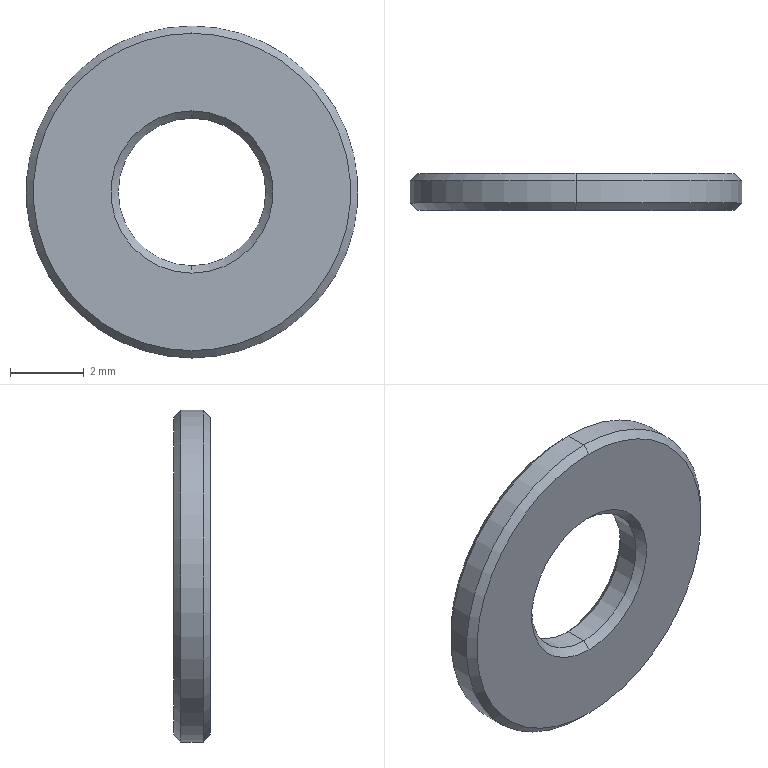Part | NX | features BREP 1 | 1 solid | 14 faces | box 9 x 1 x 9 mm | volume 49.417 mm3 | cone 8 | cylinder 4 | plane 2 | commonest cylinder face diameters 4 x2 9 x2
STEP:
#1=CARTESIAN_POINT('',(0.,1.,4.3));
#2=VERTEX_POINT('',#1);
#3=CARTESIAN_POINT('',(0.,1.,-4.3));
#4=VERTEX_POINT('',#3);
#5=CARTESIAN_POINT('',(0.,1.,0.));
#6=DIRECTION('',(0.,1.,0.));
#7=DIRECTION('',(1.,0.,0.));
#8=AXIS2_PLACEMENT_3D('',#5,#6,#7);
#9=CIRCLE('',#8,4.3);
#10=EDGE_CURVE('',#2,#4,#9,.T.);
#11=ORIENTED_EDGE('',*,*,#10,.F.);
#12=CARTESIAN_POINT('',(0.,0.8,4.5));
#13=VERTEX_POINT('',#12);
#14=CARTESIAN_POINT('',(0.,-353550.241,353555.541));
#15=DIRECTION('',(0.,0.7071,-0.7071));
#16=VECTOR('',#15,1000.);
#17=LINE('',#14,#16);
#18=EDGE_CURVE('',#13,#2,#17,.T.);
#19=ORIENTED_EDGE('',*,*,#18,.F.);
#20=CARTESIAN_POINT('',(0.,0.8,-4.5));
#21=VERTEX_POINT('',#20);
#22=CARTESIAN_POINT('',(0.,0.8,0.));
#23=DIRECTION('',(0.,-1.,0.));
#24=DIRECTION('',(1.,0.,0.));
#25=AXIS2_PLACEMENT_3D('',#22,#23,#24);
#26=CIRCLE('',#25,4.5);
#27=EDGE_CURVE('',#21,#13,#26,.T.);
#28=ORIENTED_EDGE('',*,*,#27,.F.);
#29=CARTESIAN_POINT('',(0.,-353550.241,-353555.541));
#30=DIRECTION('',(0.,0.7071,0.7071));
#31=VECTOR('',#30,1000.);
#32=LINE('',#29,#31);
#33=EDGE_CURVE('',#21,#4,#32,.T.);
#34=ORIENTED_EDGE('',*,*,#33,.T.);
#35=EDGE_LOOP('',(#11,#19,#28,#34));
#36=FACE_BOUND('',#35,.T.);
#37=CARTESIAN_POINT('',(0.,1.,0.));
#38=DIRECTION('',(0.,-1.,0.));
#39=DIRECTION('',(0.,0.,1.));
#40=AXIS2_PLACEMENT_3D('',#37,#38,#39);
#41=CONICAL_SURFACE('',#40,4.3,0.7854);
#42=ADVANCED_FACE('',(#36),#41,.T.);
#43=CARTESIAN_POINT('',(0.,1.,0.));
#44=DIRECTION('',(0.,1.,0.));
#45=DIRECTION('',(1.,0.,0.));
#46=AXIS2_PLACEMENT_3D('',#43,#44,#45);
#47=CIRCLE('',#46,4.3);
#48=EDGE_CURVE('',#4,#2,#47,.T.);
#49=ORIENTED_EDGE('',*,*,#48,.T.);
#50=ORIENTED_EDGE('',*,*,#10,.T.);
#51=EDGE_LOOP('',(#49,#50));
#52=FACE_BOUND('',#51,.T.);
#53=CARTESIAN_POINT('',(0.,1.,2.2));
#54=VERTEX_POINT('',#53);
#55=CARTESIAN_POINT('',(0.,1.,-2.2));
#56=VERTEX_POINT('',#55);
#57=CARTESIAN_POINT('',(0.,1.,2.2));
#58=CARTESIAN_POINT('',(-0.218,1.,2.2));
#59=CARTESIAN_POINT('',(-0.436,1.,2.173));
#60=CARTESIAN_POINT('',(-0.6495,1.,2.119));
#61=CARTESIAN_POINT('',(-1.059,1.,1.959));
#62=CARTESIAN_POINT('',(-1.417,1.,1.704));
#63=CARTESIAN_POINT('',(-1.579,1.,1.555));
#64=CARTESIAN_POINT('',(-1.863,1.,1.22));
#65=CARTESIAN_POINT('',(-2.057,1.,0.826));
#66=CARTESIAN_POINT('',(-2.128,1.,0.6178));
#67=CARTESIAN_POINT('',(-2.219,1.,0.1879));
#68=CARTESIAN_POINT('',(-2.202,1.,-0.251));
#69=CARTESIAN_POINT('',(-2.166,1.,-0.4684));
#70=CARTESIAN_POINT('',(-2.042,1.,-0.8896));
#71=CARTESIAN_POINT('',(-1.818,1.,-1.268));
#72=CARTESIAN_POINT('',(-1.683,1.,-1.442));
#73=CARTESIAN_POINT('',(-1.373,1.,-1.753));
#74=CARTESIAN_POINT('',(-0.9967,1.,-1.98));
#75=CARTESIAN_POINT('',(-0.7952,1.,-2.069));
#76=CARTESIAN_POINT('',(-0.5132,1.,-2.154));
#77=CARTESIAN_POINT('',(-0.223,1.,-2.191));
#78=CARTESIAN_POINT('',(-0.1486,1.,-2.197));
#79=CARTESIAN_POINT('',(-0.07431,1.,-2.2));
#80=CARTESIAN_POINT('',(0.,1.,-2.2));
#81=B_SPLINE_CURVE_WITH_KNOTS('',5,(#57,#58,#59,#60,#61,#62,#63,#64,#65,#66,#67,#68,#69,#70,#71,#72,#73,#74,#75,#76,#77,#78,#79,#80),.UNSPECIFIED.,.F.,.F.,(6,3,3,3,3,3,3,6),(0.,0.1577,0.3154,0.4731,0.6308,0.7885,0.9462,1.),.UNSPECIFIED.);
#82=EDGE_CURVE('',#54,#56,#81,.T.);
#83=ORIENTED_EDGE('',*,*,#82,.T.);
#84=CARTESIAN_POINT('',(0.,1.,-2.2));
#85=CARTESIAN_POINT('',(0.218,1.,-2.2));
#86=CARTESIAN_POINT('',(0.436,1.,-2.173));
#87=CARTESIAN_POINT('',(0.6495,1.,-2.119));
#88=CARTESIAN_POINT('',(1.059,1.,-1.959));
#89=CARTESIAN_POINT('',(1.417,1.,-1.704));
#90=CARTESIAN_POINT('',(1.579,1.,-1.555));
#91=CARTESIAN_POINT('',(1.863,1.,-1.22));
#92=CARTESIAN_POINT('',(2.057,1.,-0.826));
#93=CARTESIAN_POINT('',(2.128,1.,-0.6178));
#94=CARTESIAN_POINT('',(2.219,1.,-0.1879));
#95=CARTESIAN_POINT('',(2.202,1.,0.251));
#96=CARTESIAN_POINT('',(2.166,1.,0.4684));
#97=CARTESIAN_POINT('',(2.042,1.,0.8896));
#98=CARTESIAN_POINT('',(1.818,1.,1.268));
#99=CARTESIAN_POINT('',(1.683,1.,1.442));
#100=CARTESIAN_POINT('',(1.373,1.,1.753));
#101=CARTESIAN_POINT('',(0.9967,1.,1.98));
#102=CARTESIAN_POINT('',(0.7952,1.,2.069));
#103=CARTESIAN_POINT('',(0.5132,1.,2.154));
#104=CARTESIAN_POINT('',(0.223,1.,2.191));
#105=CARTESIAN_POINT('',(0.1486,1.,2.197));
#106=CARTESIAN_POINT('',(0.07431,1.,2.2));
#107=CARTESIAN_POINT('',(0.,1.,2.2));
#108=B_SPLINE_CURVE_WITH_KNOTS('',5,(#84,#85,#86,#87,#88,#89,#90,#91,#92,#93,#94,#95,#96,#97,#98,#99,#100,#101,#102,#103,#104,#105,#106,#107),.UNSPECIFIED.,.F.,.F.,(6,3,3,3,3,3,3,6),(0.,0.1577,0.3154,0.4731,0.6308,0.7885,0.9462,1.),.UNSPECIFIED.);
#109=EDGE_CURVE('',#56,#54,#108,.T.);
#110=ORIENTED_EDGE('',*,*,#109,.T.);
#111=EDGE_LOOP('',(#83,#110));
#112=FACE_BOUND('',#111,.T.);
#113=CARTESIAN_POINT('',(0.,1.,0.));
#114=DIRECTION('',(0.,1.,0.));
#115=DIRECTION('',(0.,0.,-1.));
#116=AXIS2_PLACEMENT_3D('',#113,#114,#115);
#117=PLANE('',#116);
#118=ADVANCED_FACE('',(#52,#112),#117,.T.);
#119=ORIENTED_EDGE('',*,*,#18,.T.);
#120=ORIENTED_EDGE('',*,*,#48,.F.);
#121=ORIENTED_EDGE('',*,*,#33,.F.);
#122=CARTESIAN_POINT('',(0.,0.8,0.));
#123=DIRECTION('',(0.,-1.,0.));
#124=DIRECTION('',(1.,0.,0.));
#125=AXIS2_PLACEMENT_3D('',#122,#123,#124);
#126=CIRCLE('',#125,4.5);
#127=EDGE_CURVE('',#13,#21,#126,.T.);
#128=ORIENTED_EDGE('',*,*,#127,.F.);
#129=EDGE_LOOP('',(#119,#120,#121,#128));
#130=FACE_BOUND('',#129,.T.);
#131=CARTESIAN_POINT('',(0.,1.,0.));
#132=DIRECTION('',(0.,-1.,0.));
#133=DIRECTION('',(0.,0.,-1.));
#134=AXIS2_PLACEMENT_3D('',#131,#132,#133);
#135=CONICAL_SURFACE('',#134,4.3,0.7854);
#136=ADVANCED_FACE('',(#130),#135,.T.);
#137=ORIENTED_EDGE('',*,*,#27,.T.);
#138=CARTESIAN_POINT('',(0.,0.2,4.5));
#139=VERTEX_POINT('',#138);
#140=CARTESIAN_POINT('',(0.,1.,4.5));
#141=DIRECTION('',(0.,1.,0.));
#142=VECTOR('',#141,1000.);
#143=LINE('',#140,#142);
#144=EDGE_CURVE('',#139,#13,#143,.T.);
#145=ORIENTED_EDGE('',*,*,#144,.F.);
#146=CARTESIAN_POINT('',(0.,0.2,-4.5));
#147=VERTEX_POINT('',#146);
#148=CARTESIAN_POINT('',(0.,0.2,0.));
#149=DIRECTION('',(0.,1.,0.));
#150=DIRECTION('',(1.,0.,0.));
#151=AXIS2_PLACEMENT_3D('',#148,#149,#150);
#152=CIRCLE('',#151,4.5);
#153=EDGE_CURVE('',#139,#147,#152,.T.);
#154=ORIENTED_EDGE('',*,*,#153,.T.);
#155=CARTESIAN_POINT('',(0.,1.,-4.5));
#156=DIRECTION('',(0.,1.,0.));
#157=VECTOR('',#156,1000.);
#158=LINE('',#155,#157);
#159=EDGE_CURVE('',#147,#21,#158,.T.);
#160=ORIENTED_EDGE('',*,*,#159,.T.);
#161=EDGE_LOOP('',(#137,#145,#154,#160));
#162=FACE_BOUND('',#161,.T.);
#163=CARTESIAN_POINT('',(0.,1.,0.));
#164=DIRECTION('',(0.,-1.,0.));
#165=DIRECTION('',(0.,0.,1.));
#166=AXIS2_PLACEMENT_3D('',#163,#164,#165);
#167=CYLINDRICAL_SURFACE('',#166,4.5);
#168=ADVANCED_FACE('',(#162),#167,.T.);
#169=CARTESIAN_POINT('',(0.,0.8,-2.));
#170=VERTEX_POINT('',#169);
#171=CARTESIAN_POINT('',(0.,0.8,2.));
#172=VERTEX_POINT('',#171);
#173=CARTESIAN_POINT('',(0.,0.8,0.));
#174=DIRECTION('',(0.,1.,0.));
#175=DIRECTION('',(1.,0.,0.));
#176=AXIS2_PLACEMENT_3D('',#173,#174,#175);
#177=CIRCLE('',#176,2.);
#178=EDGE_CURVE('',#170,#172,#177,.T.);
#179=ORIENTED_EDGE('',*,*,#178,.F.);
#180=CARTESIAN_POINT('',(0.,353553.191,-353554.391));
#181=DIRECTION('',(0.,0.7071,-0.7071));
#182=VECTOR('',#181,1000.);
#183=LINE('',#180,#182);
#184=EDGE_CURVE('',#170,#56,#183,.T.);
#185=ORIENTED_EDGE('',*,*,#184,.T.);
#186=ORIENTED_EDGE('',*,*,#82,.F.);
#187=CARTESIAN_POINT('',(0.,353553.191,353554.391));
#188=DIRECTION('',(0.,0.7071,0.7071));
#189=VECTOR('',#188,1000.);
#190=LINE('',#187,#189);
#191=EDGE_CURVE('',#172,#54,#190,.T.);
#192=ORIENTED_EDGE('',*,*,#191,.F.);
#193=EDGE_LOOP('',(#179,#185,#186,#192));
#194=FACE_BOUND('',#193,.T.);
#195=CARTESIAN_POINT('',(0.,0.8,0.));
#196=DIRECTION('',(0.,1.,0.));
#197=DIRECTION('',(0.,0.,1.));
#198=AXIS2_PLACEMENT_3D('',#195,#196,#197);
#199=CONICAL_SURFACE('',#198,2.,0.7854);
#200=ADVANCED_FACE('',(#194),#199,.F.);
#201=ORIENTED_EDGE('',*,*,#184,.F.);
#202=CARTESIAN_POINT('',(0.,0.8,0.));
#203=DIRECTION('',(0.,1.,0.));
#204=DIRECTION('',(1.,0.,0.));
#205=AXIS2_PLACEMENT_3D('',#202,#203,#204);
#206=CIRCLE('',#205,2.);
#207=EDGE_CURVE('',#172,#170,#206,.T.);
#208=ORIENTED_EDGE('',*,*,#207,.F.);
#209=ORIENTED_EDGE('',*,*,#191,.T.);
#210=ORIENTED_EDGE('',*,*,#109,.F.);
#211=EDGE_LOOP('',(#201,#208,#209,#210));
#212=FACE_BOUND('',#211,.T.);
#213=CARTESIAN_POINT('',(0.,0.8,0.));
#214=DIRECTION('',(0.,1.,0.));
#215=DIRECTION('',(0.,0.,-1.));
#216=AXIS2_PLACEMENT_3D('',#213,#214,#215);
#217=CONICAL_SURFACE('',#216,2.,0.7854);
#218=ADVANCED_FACE('',(#212),#217,.F.);
#219=ORIENTED_EDGE('',*,*,#144,.T.);
#220=ORIENTED_EDGE('',*,*,#127,.T.);
#221=ORIENTED_EDGE('',*,*,#159,.F.);
#222=CARTESIAN_POINT('',(0.,0.2,0.));
#223=DIRECTION('',(0.,1.,0.));
#224=DIRECTION('',(1.,0.,0.));
#225=AXIS2_PLACEMENT_3D('',#222,#223,#224);
#226=CIRCLE('',#225,4.5);
#227=EDGE_CURVE('',#147,#139,#226,.T.);
#228=ORIENTED_EDGE('',*,*,#227,.T.);
#229=EDGE_LOOP('',(#219,#220,#221,#228));
#230=FACE_BOUND('',#229,.T.);
#231=CARTESIAN_POINT('',(0.,1.,0.));
#232=DIRECTION('',(0.,-1.,0.));
#233=DIRECTION('',(0.,0.,-1.));
#234=AXIS2_PLACEMENT_3D('',#231,#232,#233);
#235=CYLINDRICAL_SURFACE('',#234,4.5);
#236=ADVANCED_FACE('',(#230),#235,.T.);
#237=CARTESIAN_POINT('',(0.,0.,-4.3));
#238=VERTEX_POINT('',#237);
#239=CARTESIAN_POINT('',(0.,0.,4.3));
#240=VERTEX_POINT('',#239);
#241=CARTESIAN_POINT('',(0.,0.,0.));
#242=DIRECTION('',(0.,-1.,0.));
#243=DIRECTION('',(1.,0.,0.));
#244=AXIS2_PLACEMENT_3D('',#241,#242,#243);
#245=CIRCLE('',#244,4.3);
#246=EDGE_CURVE('',#238,#240,#245,.T.);
#247=ORIENTED_EDGE('',*,*,#246,.F.);
#248=CARTESIAN_POINT('',(0.,353551.341,-353555.641));
#249=DIRECTION('',(0.,0.7071,-0.7071));
#250=VECTOR('',#249,1000.);
#251=LINE('',#248,#250);
#252=EDGE_CURVE('',#238,#147,#251,.T.);
#253=ORIENTED_EDGE('',*,*,#252,.T.);
#254=ORIENTED_EDGE('',*,*,#153,.F.);
#255=CARTESIAN_POINT('',(0.,353551.341,353555.641));
#256=DIRECTION('',(0.,0.7071,0.7071));
#257=VECTOR('',#256,1000.);
#258=LINE('',#255,#257);
#259=EDGE_CURVE('',#240,#139,#258,.T.);
#260=ORIENTED_EDGE('',*,*,#259,.F.);
#261=EDGE_LOOP('',(#247,#253,#254,#260));
#262=FACE_BOUND('',#261,.T.);
#263=CARTESIAN_POINT('',(0.,0.2,0.));
#264=DIRECTION('',(0.,1.,0.));
#265=DIRECTION('',(0.,0.,-1.));
#266=AXIS2_PLACEMENT_3D('',#263,#264,#265);
#267=CONICAL_SURFACE('',#266,4.5,0.7854);
#268=ADVANCED_FACE('',(#262),#267,.T.);
#269=ORIENTED_EDGE('',*,*,#178,.T.);
#270=CARTESIAN_POINT('',(0.,0.2,2.));
#271=VERTEX_POINT('',#270);
#272=CARTESIAN_POINT('',(0.,1.,2.));
#273=DIRECTION('',(0.,1.,0.));
#274=VECTOR('',#273,1000.);
#275=LINE('',#272,#274);
#276=EDGE_CURVE('',#271,#172,#275,.T.);
#277=ORIENTED_EDGE('',*,*,#276,.F.);
#278=CARTESIAN_POINT('',(0.,0.2,-2.));
#279=VERTEX_POINT('',#278);
#280=CARTESIAN_POINT('',(0.,0.2,0.));
#281=DIRECTION('',(0.,-1.,0.));
#282=DIRECTION('',(0.,0.,-1.));
#283=AXIS2_PLACEMENT_3D('',#280,#281,#282);
#284=CIRCLE('',#283,2.);
#285=EDGE_CURVE('',#271,#279,#284,.T.);
#286=ORIENTED_EDGE('',*,*,#285,.T.);
#287=CARTESIAN_POINT('',(0.,1.,-2.));
#288=DIRECTION('',(0.,1.,0.));
#289=VECTOR('',#288,1000.);
#290=LINE('',#287,#289);
#291=EDGE_CURVE('',#279,#170,#290,.T.);
#292=ORIENTED_EDGE('',*,*,#291,.T.);
#293=EDGE_LOOP('',(#269,#277,#286,#292));
#294=FACE_BOUND('',#293,.T.);
#295=CARTESIAN_POINT('',(0.,1.,0.));
#296=DIRECTION('',(0.,-1.,0.));
#297=DIRECTION('',(0.,0.,-1.));
#298=AXIS2_PLACEMENT_3D('',#295,#296,#297);
#299=CYLINDRICAL_SURFACE('',#298,2.);
#300=ADVANCED_FACE('',(#294),#299,.F.);
#301=ORIENTED_EDGE('',*,*,#276,.T.);
#302=ORIENTED_EDGE('',*,*,#207,.T.);
#303=ORIENTED_EDGE('',*,*,#291,.F.);
#304=CARTESIAN_POINT('',(0.,0.2,0.));
#305=DIRECTION('',(0.,-1.,0.));
#306=DIRECTION('',(1.,0.,0.));
#307=AXIS2_PLACEMENT_3D('',#304,#305,#306);
#308=CIRCLE('',#307,2.);
#309=EDGE_CURVE('',#279,#271,#308,.T.);
#310=ORIENTED_EDGE('',*,*,#309,.T.);
#311=EDGE_LOOP('',(#301,#302,#303,#310));
#312=FACE_BOUND('',#311,.T.);
#313=CARTESIAN_POINT('',(0.,1.,0.));
#314=DIRECTION('',(0.,-1.,0.));
#315=DIRECTION('',(0.,0.,1.));
#316=AXIS2_PLACEMENT_3D('',#313,#314,#315);
#317=CYLINDRICAL_SURFACE('',#316,2.);
#318=ADVANCED_FACE('',(#312),#317,.F.);
#319=ORIENTED_EDGE('',*,*,#252,.F.);
#320=CARTESIAN_POINT('',(0.,0.,0.));
#321=DIRECTION('',(0.,-1.,0.));
#322=DIRECTION('',(1.,0.,0.));
#323=AXIS2_PLACEMENT_3D('',#320,#321,#322);
#324=CIRCLE('',#323,4.3);
#325=EDGE_CURVE('',#240,#238,#324,.T.);
#326=ORIENTED_EDGE('',*,*,#325,.F.);
#327=ORIENTED_EDGE('',*,*,#259,.T.);
#328=ORIENTED_EDGE('',*,*,#227,.F.);
#329=EDGE_LOOP('',(#319,#326,#327,#328));
#330=FACE_BOUND('',#329,.T.);
#331=CARTESIAN_POINT('',(0.,0.2,0.));
#332=DIRECTION('',(0.,1.,0.));
#333=DIRECTION('',(0.,0.,1.));
#334=AXIS2_PLACEMENT_3D('',#331,#332,#333);
#335=CONICAL_SURFACE('',#334,4.5,0.7854);
#336=ADVANCED_FACE('',(#330),#335,.T.);
#337=ORIENTED_EDGE('',*,*,#325,.T.);
#338=ORIENTED_EDGE('',*,*,#246,.T.);
#339=EDGE_LOOP('',(#337,#338));
#340=FACE_BOUND('',#339,.T.);
#341=CARTESIAN_POINT('',(0.,0.,-2.2));
#342=VERTEX_POINT('',#341);
#343=CARTESIAN_POINT('',(0.,0.,2.2));
#344=VERTEX_POINT('',#343);
#345=CARTESIAN_POINT('',(0.,0.,0.));
#346=DIRECTION('',(0.,1.,0.));
#347=DIRECTION('',(1.,0.,0.));
#348=AXIS2_PLACEMENT_3D('',#345,#346,#347);
#349=CIRCLE('',#348,2.2);
#350=EDGE_CURVE('',#342,#344,#349,.T.);
#351=ORIENTED_EDGE('',*,*,#350,.T.);
#352=CARTESIAN_POINT('',(0.,0.,0.));
#353=DIRECTION('',(0.,1.,0.));
#354=DIRECTION('',(1.,0.,0.));
#355=AXIS2_PLACEMENT_3D('',#352,#353,#354);
#356=CIRCLE('',#355,2.2);
#357=EDGE_CURVE('',#344,#342,#356,.T.);
#358=ORIENTED_EDGE('',*,*,#357,.T.);
#359=EDGE_LOOP('',(#351,#358));
#360=FACE_BOUND('',#359,.T.);
#361=CARTESIAN_POINT('',(0.,0.,0.));
#362=DIRECTION('',(0.,1.,0.));
#363=DIRECTION('',(0.,0.,-1.));
#364=AXIS2_PLACEMENT_3D('',#361,#362,#363);
#365=PLANE('',#364);
#366=ADVANCED_FACE('',(#340,#360),#365,.F.);
#367=ORIENTED_EDGE('',*,*,#285,.F.);
#368=CARTESIAN_POINT('',(0.,-353552.291,353554.491));
#369=DIRECTION('',(0.,0.7071,-0.7071));
#370=VECTOR('',#369,1000.);
#371=LINE('',#368,#370);
#372=EDGE_CURVE('',#344,#271,#371,.T.);
#373=ORIENTED_EDGE('',*,*,#372,.F.);
#374=ORIENTED_EDGE('',*,*,#350,.F.);
#375=CARTESIAN_POINT('',(0.,-353552.291,-353554.491));
#376=DIRECTION('',(0.,0.7071,0.7071));
#377=VECTOR('',#376,1000.);
#378=LINE('',#375,#377);
#379=EDGE_CURVE('',#342,#279,#378,.T.);
#380=ORIENTED_EDGE('',*,*,#379,.T.);
#381=EDGE_LOOP('',(#367,#373,#374,#380));
#382=FACE_BOUND('',#381,.T.);
#383=CARTESIAN_POINT('',(0.,0.,0.));
#384=DIRECTION('',(0.,-1.,0.));
#385=DIRECTION('',(0.,0.,-1.));
#386=AXIS2_PLACEMENT_3D('',#383,#384,#385);
#387=CONICAL_SURFACE('',#386,2.2,0.7854);
#388=ADVANCED_FACE('',(#382),#387,.F.);
#389=ORIENTED_EDGE('',*,*,#372,.T.);
#390=ORIENTED_EDGE('',*,*,#309,.F.);
#391=ORIENTED_EDGE('',*,*,#379,.F.);
#392=ORIENTED_EDGE('',*,*,#357,.F.);
#393=EDGE_LOOP('',(#389,#390,#391,#392));
#394=FACE_BOUND('',#393,.T.);
#395=CARTESIAN_POINT('',(0.,0.,0.));
#396=DIRECTION('',(0.,-1.,0.));
#397=DIRECTION('',(0.,0.,1.));
#398=AXIS2_PLACEMENT_3D('',#395,#396,#397);
#399=CONICAL_SURFACE('',#398,2.2,0.7854);
#400=ADVANCED_FACE('',(#394),#399,.F.);
#401=CLOSED_SHELL('',(#42,#118,#136,#168,#200,#218,#236,#268,#300,#318,#336,#366,#388,#400));
#402=MANIFOLD_SOLID_BREP('',#401);
#403=(LENGTH_UNIT()NAMED_UNIT(*)SI_UNIT(.MILLI.,.METRE.));
#404=UNCERTAINTY_MEASURE_WITH_UNIT(LENGTH_MEASURE(0.00001),#403,'','');
#405=(NAMED_UNIT(*)PLANE_ANGLE_UNIT()SI_UNIT($,.RADIAN.));
#406=(NAMED_UNIT(*)SI_UNIT($,.STERADIAN.)SOLID_ANGLE_UNIT());
#407=(GEOMETRIC_REPRESENTATION_CONTEXT(3)GLOBAL_UNCERTAINTY_ASSIGNED_CONTEXT((#404))GLOBAL_UNIT_ASSIGNED_CONTEXT((#403,#405,#406))REPRESENTATION_CONTEXT('',''));
#408=ADVANCED_BREP_SHAPE_REPRESENTATION('',(#402),#407);